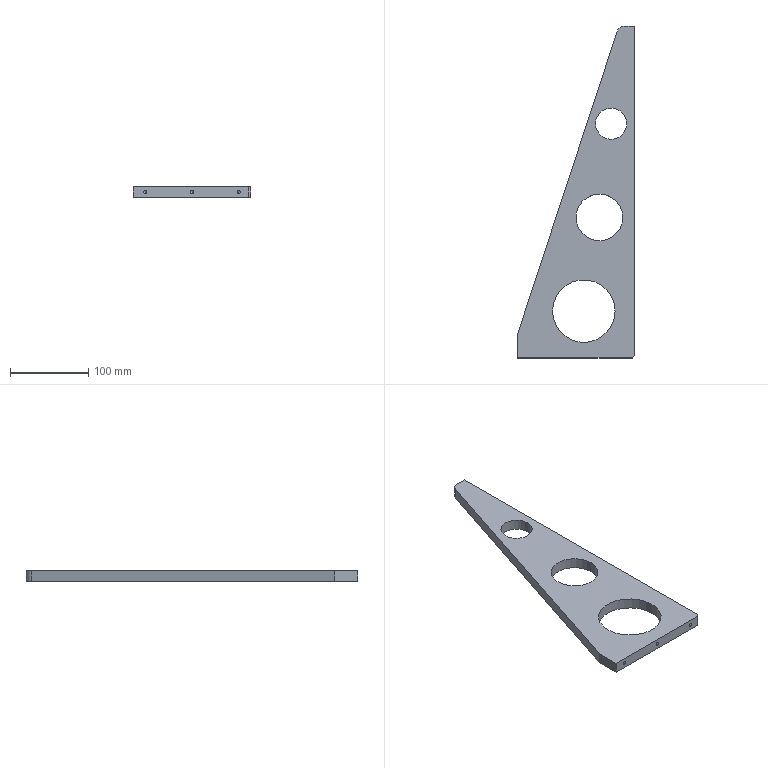Part | NX | 1 solid | 26 faces | box 150 x 425 x 14 mm | volume 403740 mm3 | cylinder 11 | plane 8 | cone 7 | commonest cylinder face diameters 4.2 x7 20 x1 40 x1 60 x1 80 x1
STEP:
#1=CARTESIAN_POINT('',(75.,-157.5,4.9));
#2=VERTEX_POINT('',#1);
#3=CARTESIAN_POINT('',(75.,-157.5,7.));
#4=DIRECTION('',(1.,0.,0.));
#5=DIRECTION('',(0.,0.,-1.));
#6=AXIS2_PLACEMENT_3D('',#3,#4,#5);
#7=CIRCLE('',#6,2.1);
#8=EDGE_CURVE('',#2,#2,#7,.T.);
#9=ORIENTED_EDGE('',*,*,#8,.F.);
#10=EDGE_LOOP('',(#9));
#11=FACE_BOUND('',#10,.T.);
#12=CARTESIAN_POINT('',(75.,-57.5,4.9));
#13=VERTEX_POINT('',#12);
#14=CARTESIAN_POINT('',(75.,-57.5,7.));
#15=DIRECTION('',(1.,0.,0.));
#16=DIRECTION('',(0.,0.,-1.));
#17=AXIS2_PLACEMENT_3D('',#14,#15,#16);
#18=CIRCLE('',#17,2.1);
#19=EDGE_CURVE('',#13,#13,#18,.T.);
#20=ORIENTED_EDGE('',*,*,#19,.F.);
#21=EDGE_LOOP('',(#20));
#22=FACE_BOUND('',#21,.T.);
#23=CARTESIAN_POINT('',(75.,42.5,4.9));
#24=VERTEX_POINT('',#23);
#25=CARTESIAN_POINT('',(75.,42.5,7.));
#26=DIRECTION('',(1.,0.,0.));
#27=DIRECTION('',(0.,0.,-1.));
#28=AXIS2_PLACEMENT_3D('',#25,#26,#27);
#29=CIRCLE('',#28,2.1);
#30=EDGE_CURVE('',#24,#24,#29,.T.);
#31=ORIENTED_EDGE('',*,*,#30,.F.);
#32=EDGE_LOOP('',(#31));
#33=FACE_BOUND('',#32,.T.);
#34=CARTESIAN_POINT('',(75.,142.5,4.9));
#35=VERTEX_POINT('',#34);
#36=CARTESIAN_POINT('',(75.,142.5,7.));
#37=DIRECTION('',(1.,0.,0.));
#38=DIRECTION('',(0.,0.,-1.));
#39=AXIS2_PLACEMENT_3D('',#36,#37,#38);
#40=CIRCLE('',#39,2.1);
#41=EDGE_CURVE('',#35,#35,#40,.T.);
#42=ORIENTED_EDGE('',*,*,#41,.F.);
#43=EDGE_LOOP('',(#42));
#44=FACE_BOUND('',#43,.T.);
#45=CARTESIAN_POINT('',(75.,-209.5,14.));
#46=VERTEX_POINT('',#45);
#47=CARTESIAN_POINT('',(75.,212.5,14.));
#48=VERTEX_POINT('',#47);
#49=CARTESIAN_POINT('',(75.,-212.5,14.));
#50=DIRECTION('',(0.,1.,0.));
#51=VECTOR('',#50,1000.);
#52=LINE('',#49,#51);
#53=EDGE_CURVE('',#46,#48,#52,.T.);
#54=ORIENTED_EDGE('',*,*,#53,.F.);
#55=CARTESIAN_POINT('',(75.,-209.5,0.));
#56=VERTEX_POINT('',#55);
#57=CARTESIAN_POINT('',(75.,-209.5,14.));
#58=DIRECTION('',(0.,0.,-1.));
#59=VECTOR('',#58,1000.);
#60=LINE('',#57,#59);
#61=EDGE_CURVE('',#46,#56,#60,.T.);
#62=ORIENTED_EDGE('',*,*,#61,.T.);
#63=CARTESIAN_POINT('',(75.,212.5,0.));
#64=VERTEX_POINT('',#63);
#65=CARTESIAN_POINT('',(75.,-212.5,0.));
#66=DIRECTION('',(0.,1.,0.));
#67=VECTOR('',#66,1000.);
#68=LINE('',#65,#67);
#69=EDGE_CURVE('',#56,#64,#68,.T.);
#70=ORIENTED_EDGE('',*,*,#69,.T.);
#71=CARTESIAN_POINT('',(75.,212.5,14.));
#72=DIRECTION('',(0.,0.,-1.));
#73=VECTOR('',#72,1000.);
#74=LINE('',#71,#73);
#75=EDGE_CURVE('',#48,#64,#74,.T.);
#76=ORIENTED_EDGE('',*,*,#75,.F.);
#77=EDGE_LOOP('',(#54,#62,#70,#76));
#78=FACE_BOUND('',#77,.T.);
#79=CARTESIAN_POINT('',(75.,-212.5,14.));
#80=DIRECTION('',(-1.,0.,0.));
#81=DIRECTION('',(0.,0.,1.));
#82=AXIS2_PLACEMENT_3D('',#79,#80,#81);
#83=PLANE('',#82);
#84=ADVANCED_FACE('',(#11,#22,#33,#44,#78),#83,.F.);
#85=CARTESIAN_POINT('',(62.237,212.5,0.));
#86=VERTEX_POINT('',#85);
#87=CARTESIAN_POINT('',(-75.,212.5,0.));
#88=DIRECTION('',(-1.,0.,0.));
#89=VECTOR('',#88,1000.);
#90=LINE('',#87,#89);
#91=EDGE_CURVE('',#64,#86,#90,.T.);
#92=ORIENTED_EDGE('',*,*,#91,.T.);
#93=CARTESIAN_POINT('',(62.237,212.5,14.));
#94=VERTEX_POINT('',#93);
#95=CARTESIAN_POINT('',(62.237,212.5,14.));
#96=DIRECTION('',(0.,0.,-1.));
#97=VECTOR('',#96,1000.);
#98=LINE('',#95,#97);
#99=EDGE_CURVE('',#86,#94,#98,.F.);
#100=ORIENTED_EDGE('',*,*,#99,.T.);
#101=CARTESIAN_POINT('',(-75.,212.5,14.));
#102=DIRECTION('',(-1.,0.,0.));
#103=VECTOR('',#102,1000.);
#104=LINE('',#101,#103);
#105=EDGE_CURVE('',#48,#94,#104,.T.);
#106=ORIENTED_EDGE('',*,*,#105,.F.);
#107=ORIENTED_EDGE('',*,*,#75,.T.);
#108=EDGE_LOOP('',(#92,#100,#106,#107));
#109=FACE_BOUND('',#108,.T.);
#110=CARTESIAN_POINT('',(-75.,212.5,14.));
#111=DIRECTION('',(0.,-1.,0.));
#112=DIRECTION('',(0.,0.,-1.));
#113=AXIS2_PLACEMENT_3D('',#110,#111,#112);
#114=PLANE('',#113);
#115=ADVANCED_FACE('',(#109),#114,.F.);
#116=CARTESIAN_POINT('',(-75.,-182.5,14.));
#117=VERTEX_POINT('',#116);
#118=CARTESIAN_POINT('',(-75.,-212.5,14.));
#119=VERTEX_POINT('',#118);
#120=CARTESIAN_POINT('',(-75.,-212.5,14.));
#121=DIRECTION('',(0.,-1.,0.));
#122=VECTOR('',#121,1000.);
#123=LINE('',#120,#122);
#124=EDGE_CURVE('',#117,#119,#123,.T.);
#125=ORIENTED_EDGE('',*,*,#124,.F.);
#126=CARTESIAN_POINT('',(-75.,-182.5,0.));
#127=VERTEX_POINT('',#126);
#128=CARTESIAN_POINT('',(-75.,-182.5,15.));
#129=DIRECTION('',(0.,0.,-1.));
#130=VECTOR('',#129,1000.);
#131=LINE('',#128,#130);
#132=EDGE_CURVE('',#117,#127,#131,.T.);
#133=ORIENTED_EDGE('',*,*,#132,.T.);
#134=CARTESIAN_POINT('',(-75.,-212.5,0.));
#135=VERTEX_POINT('',#134);
#136=CARTESIAN_POINT('',(-75.,-212.5,0.));
#137=DIRECTION('',(0.,-1.,0.));
#138=VECTOR('',#137,1000.);
#139=LINE('',#136,#138);
#140=EDGE_CURVE('',#127,#135,#139,.T.);
#141=ORIENTED_EDGE('',*,*,#140,.T.);
#142=CARTESIAN_POINT('',(-75.,-212.5,14.));
#143=DIRECTION('',(0.,0.,-1.));
#144=VECTOR('',#143,1000.);
#145=LINE('',#142,#144);
#146=EDGE_CURVE('',#119,#135,#145,.T.);
#147=ORIENTED_EDGE('',*,*,#146,.F.);
#148=EDGE_LOOP('',(#125,#133,#141,#147));
#149=FACE_BOUND('',#148,.T.);
#150=CARTESIAN_POINT('',(-75.,-212.5,14.));
#151=DIRECTION('',(1.,0.,0.));
#152=DIRECTION('',(0.,0.,-1.));
#153=AXIS2_PLACEMENT_3D('',#150,#151,#152);
#154=PLANE('',#153);
#155=ADVANCED_FACE('',(#149),#154,.F.);
#156=CARTESIAN_POINT('',(60.,-212.5,4.9));
#157=VERTEX_POINT('',#156);
#158=CARTESIAN_POINT('',(60.,-212.5,7.));
#159=DIRECTION('',(0.,-1.,0.));
#160=DIRECTION('',(0.,0.,-1.));
#161=AXIS2_PLACEMENT_3D('',#158,#159,#160);
#162=CIRCLE('',#161,2.1);
#163=EDGE_CURVE('',#157,#157,#162,.T.);
#164=ORIENTED_EDGE('',*,*,#163,.F.);
#165=EDGE_LOOP('',(#164));
#166=FACE_BOUND('',#165,.T.);
#167=CARTESIAN_POINT('',(0.,-212.5,4.9));
#168=VERTEX_POINT('',#167);
#169=CARTESIAN_POINT('',(0.,-212.5,7.));
#170=DIRECTION('',(0.,-1.,0.));
#171=DIRECTION('',(0.,0.,-1.));
#172=AXIS2_PLACEMENT_3D('',#169,#170,#171);
#173=CIRCLE('',#172,2.1);
#174=EDGE_CURVE('',#168,#168,#173,.T.);
#175=ORIENTED_EDGE('',*,*,#174,.F.);
#176=EDGE_LOOP('',(#175));
#177=FACE_BOUND('',#176,.T.);
#178=CARTESIAN_POINT('',(-60.,-212.5,4.9));
#179=VERTEX_POINT('',#178);
#180=CARTESIAN_POINT('',(-60.,-212.5,7.));
#181=DIRECTION('',(0.,-1.,0.));
#182=DIRECTION('',(0.,0.,-1.));
#183=AXIS2_PLACEMENT_3D('',#180,#181,#182);
#184=CIRCLE('',#183,2.1);
#185=EDGE_CURVE('',#179,#179,#184,.T.);
#186=ORIENTED_EDGE('',*,*,#185,.F.);
#187=EDGE_LOOP('',(#186));
#188=FACE_BOUND('',#187,.T.);
#189=CARTESIAN_POINT('',(72.,-212.5,0.));
#190=VERTEX_POINT('',#189);
#191=CARTESIAN_POINT('',(-75.,-212.5,0.));
#192=DIRECTION('',(1.,0.,0.));
#193=VECTOR('',#192,1000.);
#194=LINE('',#191,#193);
#195=EDGE_CURVE('',#135,#190,#194,.T.);
#196=ORIENTED_EDGE('',*,*,#195,.T.);
#197=CARTESIAN_POINT('',(72.,-212.5,14.));
#198=VERTEX_POINT('',#197);
#199=CARTESIAN_POINT('',(72.,-212.5,14.));
#200=DIRECTION('',(0.,0.,1.));
#201=VECTOR('',#200,1000.);
#202=LINE('',#199,#201);
#203=EDGE_CURVE('',#190,#198,#202,.T.);
#204=ORIENTED_EDGE('',*,*,#203,.T.);
#205=CARTESIAN_POINT('',(-75.,-212.5,14.));
#206=DIRECTION('',(1.,0.,0.));
#207=VECTOR('',#206,1000.);
#208=LINE('',#205,#207);
#209=EDGE_CURVE('',#119,#198,#208,.T.);
#210=ORIENTED_EDGE('',*,*,#209,.F.);
#211=ORIENTED_EDGE('',*,*,#146,.T.);
#212=EDGE_LOOP('',(#196,#204,#210,#211));
#213=FACE_BOUND('',#212,.T.);
#214=CARTESIAN_POINT('',(-75.,-212.5,14.));
#215=DIRECTION('',(0.,1.,0.));
#216=DIRECTION('',(0.,0.,1.));
#217=AXIS2_PLACEMENT_3D('',#214,#215,#216);
#218=PLANE('',#217);
#219=ADVANCED_FACE('',(#166,#177,#188,#213),#218,.F.);
#220=CARTESIAN_POINT('',(65.,87.5,14.));
#221=VERTEX_POINT('',#220);
#222=CARTESIAN_POINT('',(45.,87.5,14.));
#223=DIRECTION('',(0.,0.,1.));
#224=DIRECTION('',(1.,0.,0.));
#225=AXIS2_PLACEMENT_3D('',#222,#223,#224);
#226=CIRCLE('',#225,20.);
#227=EDGE_CURVE('',#221,#221,#226,.T.);
#228=ORIENTED_EDGE('',*,*,#227,.F.);
#229=EDGE_LOOP('',(#228));
#230=FACE_BOUND('',#229,.T.);
#231=CARTESIAN_POINT('',(60.,-32.5,14.));
#232=VERTEX_POINT('',#231);
#233=CARTESIAN_POINT('',(30.,-32.5,14.));
#234=DIRECTION('',(0.,0.,1.));
#235=DIRECTION('',(1.,0.,0.));
#236=AXIS2_PLACEMENT_3D('',#233,#234,#235);
#237=CIRCLE('',#236,30.);
#238=EDGE_CURVE('',#232,#232,#237,.T.);
#239=ORIENTED_EDGE('',*,*,#238,.F.);
#240=EDGE_LOOP('',(#239));
#241=FACE_BOUND('',#240,.T.);
#242=CARTESIAN_POINT('',(50.,-152.5,14.));
#243=VERTEX_POINT('',#242);
#244=CARTESIAN_POINT('',(10.,-152.5,14.));
#245=DIRECTION('',(0.,0.,1.));
#246=DIRECTION('',(1.,0.,0.));
#247=AXIS2_PLACEMENT_3D('',#244,#245,#246);
#248=CIRCLE('',#247,40.);
#249=EDGE_CURVE('',#243,#243,#248,.T.);
#250=ORIENTED_EDGE('',*,*,#249,.F.);
#251=EDGE_LOOP('',(#250));
#252=FACE_BOUND('',#251,.T.);
#253=ORIENTED_EDGE('',*,*,#209,.T.);
#254=CARTESIAN_POINT('',(75.,-209.5,14.));
#255=DIRECTION('',(-0.7071,-0.7071,0.));
#256=VECTOR('',#255,1000.);
#257=LINE('',#254,#256);
#258=EDGE_CURVE('',#198,#46,#257,.F.);
#259=ORIENTED_EDGE('',*,*,#258,.T.);
#260=ORIENTED_EDGE('',*,*,#53,.T.);
#261=ORIENTED_EDGE('',*,*,#105,.T.);
#262=CARTESIAN_POINT('',(52.738,205.626,14.));
#263=VERTEX_POINT('',#262);
#264=CARTESIAN_POINT('',(62.237,202.5,14.));
#265=DIRECTION('',(0.,0.,-1.));
#266=DIRECTION('',(-1.,0.,0.));
#267=AXIS2_PLACEMENT_3D('',#264,#265,#266);
#268=CIRCLE('',#267,10.);
#269=EDGE_CURVE('',#94,#263,#268,.F.);
#270=ORIENTED_EDGE('',*,*,#269,.T.);
#271=CARTESIAN_POINT('',(56.955,218.439,14.));
#272=DIRECTION('',(-0.3126,-0.9499,0.));
#273=VECTOR('',#272,1000.);
#274=LINE('',#271,#273);
#275=EDGE_CURVE('',#263,#117,#274,.T.);
#276=ORIENTED_EDGE('',*,*,#275,.T.);
#277=ORIENTED_EDGE('',*,*,#124,.T.);
#278=EDGE_LOOP('',(#253,#259,#260,#261,#270,#276,#277));
#279=FACE_BOUND('',#278,.T.);
#280=CARTESIAN_POINT('',(75.,212.5,14.));
#281=DIRECTION('',(0.,0.,-1.));
#282=DIRECTION('',(-1.,0.,0.));
#283=AXIS2_PLACEMENT_3D('',#280,#281,#282);
#284=PLANE('',#283);
#285=ADVANCED_FACE('',(#230,#241,#252,#279),#284,.F.);
#286=CARTESIAN_POINT('',(65.,87.5,0.));
#287=VERTEX_POINT('',#286);
#288=CARTESIAN_POINT('',(45.,87.5,0.));
#289=DIRECTION('',(0.,0.,1.));
#290=DIRECTION('',(1.,0.,0.));
#291=AXIS2_PLACEMENT_3D('',#288,#289,#290);
#292=CIRCLE('',#291,20.);
#293=EDGE_CURVE('',#287,#287,#292,.T.);
#294=ORIENTED_EDGE('',*,*,#293,.T.);
#295=EDGE_LOOP('',(#294));
#296=FACE_BOUND('',#295,.T.);
#297=CARTESIAN_POINT('',(60.,-32.5,0.));
#298=VERTEX_POINT('',#297);
#299=CARTESIAN_POINT('',(30.,-32.5,0.));
#300=DIRECTION('',(0.,0.,1.));
#301=DIRECTION('',(1.,0.,0.));
#302=AXIS2_PLACEMENT_3D('',#299,#300,#301);
#303=CIRCLE('',#302,30.);
#304=EDGE_CURVE('',#298,#298,#303,.T.);
#305=ORIENTED_EDGE('',*,*,#304,.T.);
#306=EDGE_LOOP('',(#305));
#307=FACE_BOUND('',#306,.T.);
#308=CARTESIAN_POINT('',(50.,-152.5,0.));
#309=VERTEX_POINT('',#308);
#310=CARTESIAN_POINT('',(10.,-152.5,0.));
#311=DIRECTION('',(0.,0.,1.));
#312=DIRECTION('',(1.,0.,0.));
#313=AXIS2_PLACEMENT_3D('',#310,#311,#312);
#314=CIRCLE('',#313,40.);
#315=EDGE_CURVE('',#309,#309,#314,.T.);
#316=ORIENTED_EDGE('',*,*,#315,.T.);
#317=EDGE_LOOP('',(#316));
#318=FACE_BOUND('',#317,.T.);
#319=ORIENTED_EDGE('',*,*,#69,.F.);
#320=CARTESIAN_POINT('',(286.,1.5,0.));
#321=DIRECTION('',(0.7071,0.7071,0.));
#322=VECTOR('',#321,1000.);
#323=LINE('',#320,#322);
#324=EDGE_CURVE('',#56,#190,#323,.F.);
#325=ORIENTED_EDGE('',*,*,#324,.T.);
#326=ORIENTED_EDGE('',*,*,#195,.F.);
#327=ORIENTED_EDGE('',*,*,#140,.F.);
#328=CARTESIAN_POINT('',(52.738,205.626,0.));
#329=VERTEX_POINT('',#328);
#330=CARTESIAN_POINT('',(55.,212.5,0.));
#331=DIRECTION('',(-0.3126,-0.9499,0.));
#332=VECTOR('',#331,1000.);
#333=LINE('',#330,#332);
#334=EDGE_CURVE('',#329,#127,#333,.T.);
#335=ORIENTED_EDGE('',*,*,#334,.F.);
#336=CARTESIAN_POINT('',(62.237,202.5,0.));
#337=DIRECTION('',(0.,0.,-1.));
#338=DIRECTION('',(-1.,0.,0.));
#339=AXIS2_PLACEMENT_3D('',#336,#337,#338);
#340=CIRCLE('',#339,10.);
#341=EDGE_CURVE('',#329,#86,#340,.T.);
#342=ORIENTED_EDGE('',*,*,#341,.T.);
#343=ORIENTED_EDGE('',*,*,#91,.F.);
#344=EDGE_LOOP('',(#319,#325,#326,#327,#335,#342,#343));
#345=FACE_BOUND('',#344,.T.);
#346=CARTESIAN_POINT('',(75.,212.5,0.));
#347=DIRECTION('',(0.,0.,-1.));
#348=DIRECTION('',(-1.,0.,0.));
#349=AXIS2_PLACEMENT_3D('',#346,#347,#348);
#350=PLANE('',#349);
#351=ADVANCED_FACE('',(#296,#307,#318,#345),#350,.T.);
#352=ORIENTED_EDGE('',*,*,#275,.F.);
#353=CARTESIAN_POINT('',(52.738,205.626,15.));
#354=DIRECTION('',(0.,0.,-1.));
#355=VECTOR('',#354,1000.);
#356=LINE('',#353,#355);
#357=EDGE_CURVE('',#263,#329,#356,.T.);
#358=ORIENTED_EDGE('',*,*,#357,.T.);
#359=ORIENTED_EDGE('',*,*,#334,.T.);
#360=ORIENTED_EDGE('',*,*,#132,.F.);
#361=EDGE_LOOP('',(#352,#358,#359,#360));
#362=FACE_BOUND('',#361,.T.);
#363=CARTESIAN_POINT('',(55.,212.5,15.));
#364=DIRECTION('',(0.9499,-0.3126,0.));
#365=DIRECTION('',(0.3126,0.9499,0.));
#366=AXIS2_PLACEMENT_3D('',#363,#364,#365);
#367=PLANE('',#366);
#368=ADVANCED_FACE('',(#362),#367,.F.);
#369=CARTESIAN_POINT('',(-60.,-193.838,7.));
#370=VERTEX_POINT('',#369);
#371=VERTEX_LOOP('',#370);
#372=FACE_BOUND('',#371,.T.);
#373=CARTESIAN_POINT('',(-60.,-195.1,4.9));
#374=VERTEX_POINT('',#373);
#375=CARTESIAN_POINT('',(-60.,-195.1,7.));
#376=DIRECTION('',(0.,-1.,0.));
#377=DIRECTION('',(0.,0.,-1.));
#378=AXIS2_PLACEMENT_3D('',#375,#376,#377);
#379=CIRCLE('',#378,2.1);
#380=EDGE_CURVE('',#374,#374,#379,.T.);
#381=ORIENTED_EDGE('',*,*,#380,.T.);
#382=EDGE_LOOP('',(#381));
#383=FACE_BOUND('',#382,.T.);
#384=CARTESIAN_POINT('',(-60.,-195.1,7.));
#385=DIRECTION('',(0.,-1.,0.));
#386=DIRECTION('',(0.,0.,-1.));
#387=AXIS2_PLACEMENT_3D('',#384,#385,#386);
#388=CONICAL_SURFACE('',#387,2.1,1.03);
#389=ADVANCED_FACE('',(#372,#383),#388,.F.);
#390=ORIENTED_EDGE('',*,*,#380,.F.);
#391=EDGE_LOOP('',(#390));
#392=FACE_BOUND('',#391,.T.);
#393=ORIENTED_EDGE('',*,*,#185,.T.);
#394=EDGE_LOOP('',(#393));
#395=FACE_BOUND('',#394,.T.);
#396=CARTESIAN_POINT('',(-60.,-212.5,7.));
#397=DIRECTION('',(0.,-1.,0.));
#398=DIRECTION('',(0.,0.,-1.));
#399=AXIS2_PLACEMENT_3D('',#396,#397,#398);
#400=CYLINDRICAL_SURFACE('',#399,2.1);
#401=ADVANCED_FACE('',(#392,#395),#400,.F.);
#402=CARTESIAN_POINT('',(0.,-193.838,7.));
#403=VERTEX_POINT('',#402);
#404=VERTEX_LOOP('',#403);
#405=FACE_BOUND('',#404,.T.);
#406=CARTESIAN_POINT('',(0.,-195.1,4.9));
#407=VERTEX_POINT('',#406);
#408=CARTESIAN_POINT('',(0.,-195.1,7.));
#409=DIRECTION('',(0.,-1.,0.));
#410=DIRECTION('',(0.,0.,-1.));
#411=AXIS2_PLACEMENT_3D('',#408,#409,#410);
#412=CIRCLE('',#411,2.1);
#413=EDGE_CURVE('',#407,#407,#412,.T.);
#414=ORIENTED_EDGE('',*,*,#413,.T.);
#415=EDGE_LOOP('',(#414));
#416=FACE_BOUND('',#415,.T.);
#417=CARTESIAN_POINT('',(0.,-195.1,7.));
#418=DIRECTION('',(0.,-1.,0.));
#419=DIRECTION('',(0.,0.,-1.));
#420=AXIS2_PLACEMENT_3D('',#417,#418,#419);
#421=CONICAL_SURFACE('',#420,2.1,1.03);
#422=ADVANCED_FACE('',(#405,#416),#421,.F.);
#423=ORIENTED_EDGE('',*,*,#413,.F.);
#424=EDGE_LOOP('',(#423));
#425=FACE_BOUND('',#424,.T.);
#426=ORIENTED_EDGE('',*,*,#174,.T.);
#427=EDGE_LOOP('',(#426));
#428=FACE_BOUND('',#427,.T.);
#429=CARTESIAN_POINT('',(0.,-212.5,7.));
#430=DIRECTION('',(0.,-1.,0.));
#431=DIRECTION('',(0.,0.,-1.));
#432=AXIS2_PLACEMENT_3D('',#429,#430,#431);
#433=CYLINDRICAL_SURFACE('',#432,2.1);
#434=ADVANCED_FACE('',(#425,#428),#433,.F.);
#435=CARTESIAN_POINT('',(60.,-193.838,7.));
#436=VERTEX_POINT('',#435);
#437=VERTEX_LOOP('',#436);
#438=FACE_BOUND('',#437,.T.);
#439=CARTESIAN_POINT('',(60.,-195.1,4.9));
#440=VERTEX_POINT('',#439);
#441=CARTESIAN_POINT('',(60.,-195.1,7.));
#442=DIRECTION('',(0.,-1.,0.));
#443=DIRECTION('',(0.,0.,-1.));
#444=AXIS2_PLACEMENT_3D('',#441,#442,#443);
#445=CIRCLE('',#444,2.1);
#446=EDGE_CURVE('',#440,#440,#445,.T.);
#447=ORIENTED_EDGE('',*,*,#446,.T.);
#448=EDGE_LOOP('',(#447));
#449=FACE_BOUND('',#448,.T.);
#450=CARTESIAN_POINT('',(60.,-195.1,7.));
#451=DIRECTION('',(0.,-1.,0.));
#452=DIRECTION('',(0.,0.,-1.));
#453=AXIS2_PLACEMENT_3D('',#450,#451,#452);
#454=CONICAL_SURFACE('',#453,2.1,1.03);
#455=ADVANCED_FACE('',(#438,#449),#454,.F.);
#456=ORIENTED_EDGE('',*,*,#446,.F.);
#457=EDGE_LOOP('',(#456));
#458=FACE_BOUND('',#457,.T.);
#459=ORIENTED_EDGE('',*,*,#163,.T.);
#460=EDGE_LOOP('',(#459));
#461=FACE_BOUND('',#460,.T.);
#462=CARTESIAN_POINT('',(60.,-212.5,7.));
#463=DIRECTION('',(0.,-1.,0.));
#464=DIRECTION('',(0.,0.,-1.));
#465=AXIS2_PLACEMENT_3D('',#462,#463,#464);
#466=CYLINDRICAL_SURFACE('',#465,2.1);
#467=ADVANCED_FACE('',(#458,#461),#466,.F.);
#468=CARTESIAN_POINT('',(59.338,142.5,7.));
#469=VERTEX_POINT('',#468);
#470=VERTEX_LOOP('',#469);
#471=FACE_BOUND('',#470,.T.);
#472=CARTESIAN_POINT('',(60.6,142.5,4.9));
#473=VERTEX_POINT('',#472);
#474=CARTESIAN_POINT('',(60.6,142.5,7.));
#475=DIRECTION('',(1.,0.,0.));
#476=DIRECTION('',(0.,0.,-1.));
#477=AXIS2_PLACEMENT_3D('',#474,#475,#476);
#478=CIRCLE('',#477,2.1);
#479=EDGE_CURVE('',#473,#473,#478,.T.);
#480=ORIENTED_EDGE('',*,*,#479,.T.);
#481=EDGE_LOOP('',(#480));
#482=FACE_BOUND('',#481,.T.);
#483=CARTESIAN_POINT('',(60.6,142.5,7.));
#484=DIRECTION('',(1.,0.,0.));
#485=DIRECTION('',(0.,0.,-1.));
#486=AXIS2_PLACEMENT_3D('',#483,#484,#485);
#487=CONICAL_SURFACE('',#486,2.1,1.03);
#488=ADVANCED_FACE('',(#471,#482),#487,.F.);
#489=ORIENTED_EDGE('',*,*,#479,.F.);
#490=EDGE_LOOP('',(#489));
#491=FACE_BOUND('',#490,.T.);
#492=ORIENTED_EDGE('',*,*,#41,.T.);
#493=EDGE_LOOP('',(#492));
#494=FACE_BOUND('',#493,.T.);
#495=CARTESIAN_POINT('',(75.,142.5,7.));
#496=DIRECTION('',(1.,0.,0.));
#497=DIRECTION('',(0.,0.,-1.));
#498=AXIS2_PLACEMENT_3D('',#495,#496,#497);
#499=CYLINDRICAL_SURFACE('',#498,2.1);
#500=ADVANCED_FACE('',(#491,#494),#499,.F.);
#501=CARTESIAN_POINT('',(59.338,42.5,7.));
#502=VERTEX_POINT('',#501);
#503=VERTEX_LOOP('',#502);
#504=FACE_BOUND('',#503,.T.);
#505=CARTESIAN_POINT('',(60.6,42.5,4.9));
#506=VERTEX_POINT('',#505);
#507=CARTESIAN_POINT('',(60.6,42.5,7.));
#508=DIRECTION('',(1.,0.,0.));
#509=DIRECTION('',(0.,0.,-1.));
#510=AXIS2_PLACEMENT_3D('',#507,#508,#509);
#511=CIRCLE('',#510,2.1);
#512=EDGE_CURVE('',#506,#506,#511,.T.);
#513=ORIENTED_EDGE('',*,*,#512,.T.);
#514=EDGE_LOOP('',(#513));
#515=FACE_BOUND('',#514,.T.);
#516=CARTESIAN_POINT('',(60.6,42.5,7.));
#517=DIRECTION('',(1.,0.,0.));
#518=DIRECTION('',(0.,0.,-1.));
#519=AXIS2_PLACEMENT_3D('',#516,#517,#518);
#520=CONICAL_SURFACE('',#519,2.1,1.03);
#521=ADVANCED_FACE('',(#504,#515),#520,.F.);
#522=ORIENTED_EDGE('',*,*,#512,.F.);
#523=EDGE_LOOP('',(#522));
#524=FACE_BOUND('',#523,.T.);
#525=ORIENTED_EDGE('',*,*,#30,.T.);
#526=EDGE_LOOP('',(#525));
#527=FACE_BOUND('',#526,.T.);
#528=CARTESIAN_POINT('',(75.,42.5,7.));
#529=DIRECTION('',(1.,0.,0.));
#530=DIRECTION('',(0.,0.,-1.));
#531=AXIS2_PLACEMENT_3D('',#528,#529,#530);
#532=CYLINDRICAL_SURFACE('',#531,2.1);
#533=ADVANCED_FACE('',(#524,#527),#532,.F.);
#534=CARTESIAN_POINT('',(59.338,-57.5,7.));
#535=VERTEX_POINT('',#534);
#536=VERTEX_LOOP('',#535);
#537=FACE_BOUND('',#536,.T.);
#538=CARTESIAN_POINT('',(60.6,-57.5,4.9));
#539=VERTEX_POINT('',#538);
#540=CARTESIAN_POINT('',(60.6,-57.5,7.));
#541=DIRECTION('',(1.,0.,0.));
#542=DIRECTION('',(0.,0.,-1.));
#543=AXIS2_PLACEMENT_3D('',#540,#541,#542);
#544=CIRCLE('',#543,2.1);
#545=EDGE_CURVE('',#539,#539,#544,.T.);
#546=ORIENTED_EDGE('',*,*,#545,.T.);
#547=EDGE_LOOP('',(#546));
#548=FACE_BOUND('',#547,.T.);
#549=CARTESIAN_POINT('',(60.6,-57.5,7.));
#550=DIRECTION('',(1.,0.,0.));
#551=DIRECTION('',(0.,0.,-1.));
#552=AXIS2_PLACEMENT_3D('',#549,#550,#551);
#553=CONICAL_SURFACE('',#552,2.1,1.03);
#554=ADVANCED_FACE('',(#537,#548),#553,.F.);
#555=ORIENTED_EDGE('',*,*,#545,.F.);
#556=EDGE_LOOP('',(#555));
#557=FACE_BOUND('',#556,.T.);
#558=ORIENTED_EDGE('',*,*,#19,.T.);
#559=EDGE_LOOP('',(#558));
#560=FACE_BOUND('',#559,.T.);
#561=CARTESIAN_POINT('',(75.,-57.5,7.));
#562=DIRECTION('',(1.,0.,0.));
#563=DIRECTION('',(0.,0.,-1.));
#564=AXIS2_PLACEMENT_3D('',#561,#562,#563);
#565=CYLINDRICAL_SURFACE('',#564,2.1);
#566=ADVANCED_FACE('',(#557,#560),#565,.F.);
#567=CARTESIAN_POINT('',(59.338,-157.5,7.));
#568=VERTEX_POINT('',#567);
#569=VERTEX_LOOP('',#568);
#570=FACE_BOUND('',#569,.T.);
#571=CARTESIAN_POINT('',(60.6,-157.5,4.9));
#572=VERTEX_POINT('',#571);
#573=CARTESIAN_POINT('',(60.6,-157.5,7.));
#574=DIRECTION('',(1.,0.,0.));
#575=DIRECTION('',(0.,0.,-1.));
#576=AXIS2_PLACEMENT_3D('',#573,#574,#575);
#577=CIRCLE('',#576,2.1);
#578=EDGE_CURVE('',#572,#572,#577,.T.);
#579=ORIENTED_EDGE('',*,*,#578,.T.);
#580=EDGE_LOOP('',(#579));
#581=FACE_BOUND('',#580,.T.);
#582=CARTESIAN_POINT('',(60.6,-157.5,7.));
#583=DIRECTION('',(1.,0.,0.));
#584=DIRECTION('',(0.,0.,-1.));
#585=AXIS2_PLACEMENT_3D('',#582,#583,#584);
#586=CONICAL_SURFACE('',#585,2.1,1.03);
#587=ADVANCED_FACE('',(#570,#581),#586,.F.);
#588=ORIENTED_EDGE('',*,*,#578,.F.);
#589=EDGE_LOOP('',(#588));
#590=FACE_BOUND('',#589,.T.);
#591=ORIENTED_EDGE('',*,*,#8,.T.);
#592=EDGE_LOOP('',(#591));
#593=FACE_BOUND('',#592,.T.);
#594=CARTESIAN_POINT('',(75.,-157.5,7.));
#595=DIRECTION('',(1.,0.,0.));
#596=DIRECTION('',(0.,0.,-1.));
#597=AXIS2_PLACEMENT_3D('',#594,#595,#596);
#598=CYLINDRICAL_SURFACE('',#597,2.1);
#599=ADVANCED_FACE('',(#590,#593),#598,.F.);
#600=ORIENTED_EDGE('',*,*,#315,.F.);
#601=EDGE_LOOP('',(#600));
#602=FACE_BOUND('',#601,.T.);
#603=ORIENTED_EDGE('',*,*,#249,.T.);
#604=EDGE_LOOP('',(#603));
#605=FACE_BOUND('',#604,.T.);
#606=CARTESIAN_POINT('',(10.,-152.5,0.));
#607=DIRECTION('',(0.,0.,1.));
#608=DIRECTION('',(1.,0.,0.));
#609=AXIS2_PLACEMENT_3D('',#606,#607,#608);
#610=CYLINDRICAL_SURFACE('',#609,40.);
#611=ADVANCED_FACE('',(#602,#605),#610,.F.);
#612=ORIENTED_EDGE('',*,*,#304,.F.);
#613=EDGE_LOOP('',(#612));
#614=FACE_BOUND('',#613,.T.);
#615=ORIENTED_EDGE('',*,*,#238,.T.);
#616=EDGE_LOOP('',(#615));
#617=FACE_BOUND('',#616,.T.);
#618=CARTESIAN_POINT('',(30.,-32.5,0.));
#619=DIRECTION('',(0.,0.,1.));
#620=DIRECTION('',(1.,0.,0.));
#621=AXIS2_PLACEMENT_3D('',#618,#619,#620);
#622=CYLINDRICAL_SURFACE('',#621,30.);
#623=ADVANCED_FACE('',(#614,#617),#622,.F.);
#624=ORIENTED_EDGE('',*,*,#293,.F.);
#625=EDGE_LOOP('',(#624));
#626=FACE_BOUND('',#625,.T.);
#627=ORIENTED_EDGE('',*,*,#227,.T.);
#628=EDGE_LOOP('',(#627));
#629=FACE_BOUND('',#628,.T.);
#630=CARTESIAN_POINT('',(45.,87.5,0.));
#631=DIRECTION('',(0.,0.,1.));
#632=DIRECTION('',(1.,0.,0.));
#633=AXIS2_PLACEMENT_3D('',#630,#631,#632);
#634=CYLINDRICAL_SURFACE('',#633,20.);
#635=ADVANCED_FACE('',(#626,#629),#634,.F.);
#636=ORIENTED_EDGE('',*,*,#269,.F.);
#637=ORIENTED_EDGE('',*,*,#99,.F.);
#638=ORIENTED_EDGE('',*,*,#341,.F.);
#639=ORIENTED_EDGE('',*,*,#357,.F.);
#640=EDGE_LOOP('',(#636,#637,#638,#639));
#641=FACE_BOUND('',#640,.T.);
#642=CARTESIAN_POINT('',(62.237,202.5,15.));
#643=DIRECTION('',(0.,0.,-1.));
#644=DIRECTION('',(-1.,0.,0.));
#645=AXIS2_PLACEMENT_3D('',#642,#643,#644);
#646=CYLINDRICAL_SURFACE('',#645,10.);
#647=ADVANCED_FACE('',(#641),#646,.T.);
#648=ORIENTED_EDGE('',*,*,#258,.F.);
#649=ORIENTED_EDGE('',*,*,#203,.F.);
#650=ORIENTED_EDGE('',*,*,#324,.F.);
#651=ORIENTED_EDGE('',*,*,#61,.F.);
#652=EDGE_LOOP('',(#648,#649,#650,#651));
#653=FACE_BOUND('',#652,.T.);
#654=CARTESIAN_POINT('',(75.,-209.5,14.));
#655=DIRECTION('',(-0.7071,0.7071,0.));
#656=DIRECTION('',(0.,0.,-1.));
#657=AXIS2_PLACEMENT_3D('',#654,#655,#656);
#658=PLANE('',#657);
#659=ADVANCED_FACE('',(#653),#658,.F.);
#660=CLOSED_SHELL('',(#84,#115,#155,#219,#285,#351,#368,#389,#401,#422,#434,#455,#467,#488,#500,#521,#533,#554,#566,#587,#599,#611,#623,#635,#647,#659));
#661=MANIFOLD_SOLID_BREP('',#660);
#662=(LENGTH_UNIT()NAMED_UNIT(*)SI_UNIT(.MILLI.,.METRE.));
#663=UNCERTAINTY_MEASURE_WITH_UNIT(LENGTH_MEASURE(0.00001),#662,'','');
#664=(NAMED_UNIT(*)PLANE_ANGLE_UNIT()SI_UNIT($,.RADIAN.));
#665=(NAMED_UNIT(*)SI_UNIT($,.STERADIAN.)SOLID_ANGLE_UNIT());
#666=(GEOMETRIC_REPRESENTATION_CONTEXT(3)GLOBAL_UNCERTAINTY_ASSIGNED_CONTEXT((#663))GLOBAL_UNIT_ASSIGNED_CONTEXT((#662,#664,#665))REPRESENTATION_CONTEXT('',''));
#667=ADVANCED_BREP_SHAPE_REPRESENTATION('',(#661),#666);